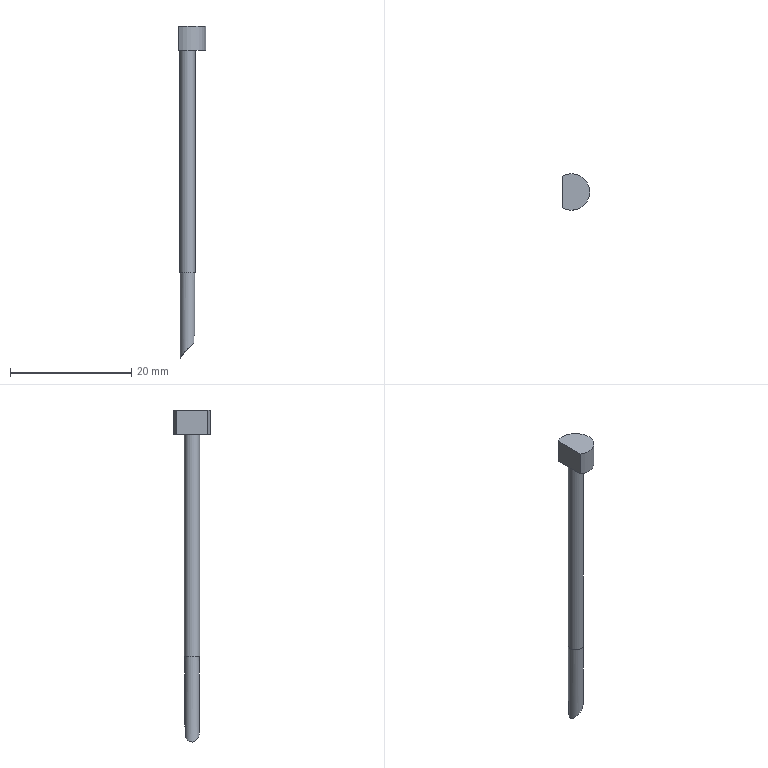Part | NX | features solid 2 | 1 solid | 10 faces | box 4.5 x 6 x 54.716 mm | volume 326.28 mm3 | cylinder 6 | plane 4 | commonest cylinder face diameters 24.622 x2 2.412 x1 2.5 x1 6 x1 26.633 x1
STEP:
#1=CARTESIAN_POINT('',(-10.383,6.106,66.5));
#2=VERTEX_POINT('',#1);
#3=CARTESIAN_POINT('',(-10.383,6.106,70.5));
#4=VERTEX_POINT('',#3);
#5=CARTESIAN_POINT('',(-10.383,6.106,66.5));
#6=DIRECTION('',(0.,0.,1.));
#7=VECTOR('',#6,1000.);
#8=LINE('',#5,#7);
#9=EDGE_CURVE('',#2,#4,#8,.T.);
#10=ORIENTED_EDGE('',*,*,#9,.F.);
#11=CARTESIAN_POINT('',(-10.383,11.303,66.5));
#12=VERTEX_POINT('',#11);
#13=CARTESIAN_POINT('',(-8.883,8.704,66.5));
#14=DIRECTION('',(0.,0.,-1.));
#15=DIRECTION('',(-1.,0.,0.));
#16=AXIS2_PLACEMENT_3D('',#13,#14,#15);
#17=CIRCLE('',#16,3.);
#18=EDGE_CURVE('',#12,#2,#17,.T.);
#19=ORIENTED_EDGE('',*,*,#18,.F.);
#20=CARTESIAN_POINT('',(-10.383,11.303,70.5));
#21=VERTEX_POINT('',#20);
#22=CARTESIAN_POINT('',(-10.383,11.303,66.5));
#23=DIRECTION('',(0.,0.,1.));
#24=VECTOR('',#23,1000.);
#25=LINE('',#22,#24);
#26=EDGE_CURVE('',#21,#12,#25,.F.);
#27=ORIENTED_EDGE('',*,*,#26,.F.);
#28=CARTESIAN_POINT('',(-8.883,8.704,70.5));
#29=DIRECTION('',(0.,0.,-1.));
#30=DIRECTION('',(-1.,0.,0.));
#31=AXIS2_PLACEMENT_3D('',#28,#29,#30);
#32=CIRCLE('',#31,3.);
#33=EDGE_CURVE('',#21,#4,#32,.T.);
#34=ORIENTED_EDGE('',*,*,#33,.T.);
#35=EDGE_LOOP('',(#10,#19,#27,#34));
#36=FACE_BOUND('',#35,.T.);
#37=CARTESIAN_POINT('',(-8.883,8.704,66.5));
#38=DIRECTION('',(0.,0.,1.));
#39=DIRECTION('',(1.,0.,0.));
#40=AXIS2_PLACEMENT_3D('',#37,#38,#39);
#41=CYLINDRICAL_SURFACE('',#40,3.);
#42=ADVANCED_FACE('',(#36),#41,.T.);
#43=CARTESIAN_POINT('',(-10.133,8.704,66.5));
#44=VERTEX_POINT('',#43);
#45=CARTESIAN_POINT('',(-8.883,8.704,66.5));
#46=DIRECTION('',(0.,0.,-1.));
#47=DIRECTION('',(-1.,0.,0.));
#48=AXIS2_PLACEMENT_3D('',#45,#46,#47);
#49=CIRCLE('',#48,1.25);
#50=EDGE_CURVE('',#44,#44,#49,.F.);
#51=ORIENTED_EDGE('',*,*,#50,.T.);
#52=EDGE_LOOP('',(#51));
#53=FACE_BOUND('',#52,.T.);
#54=ORIENTED_EDGE('',*,*,#18,.T.);
#55=CARTESIAN_POINT('',(-10.383,8.704,66.5));
#56=DIRECTION('',(0.,1.,0.));
#57=VECTOR('',#56,1000.);
#58=LINE('',#55,#57);
#59=EDGE_CURVE('',#2,#12,#58,.T.);
#60=ORIENTED_EDGE('',*,*,#59,.T.);
#61=EDGE_LOOP('',(#54,#60));
#62=FACE_BOUND('',#61,.T.);
#63=CARTESIAN_POINT('',(-8.883,8.704,66.5));
#64=DIRECTION('',(0.,0.,-1.));
#65=DIRECTION('',(-1.,0.,0.));
#66=AXIS2_PLACEMENT_3D('',#63,#64,#65);
#67=PLANE('',#66);
#68=ADVANCED_FACE('',(#53,#62),#67,.T.);
#69=ORIENTED_EDGE('',*,*,#33,.F.);
#70=CARTESIAN_POINT('',(-10.383,0.,70.5));
#71=DIRECTION('',(0.,-1.,0.));
#72=VECTOR('',#71,1000.);
#73=LINE('',#70,#72);
#74=EDGE_CURVE('',#4,#21,#73,.F.);
#75=ORIENTED_EDGE('',*,*,#74,.F.);
#76=EDGE_LOOP('',(#69,#75));
#77=FACE_BOUND('',#76,.T.);
#78=CARTESIAN_POINT('',(0.,0.,70.5));
#79=DIRECTION('',(0.,0.,1.));
#80=DIRECTION('',(1.,0.,0.));
#81=AXIS2_PLACEMENT_3D('',#78,#79,#80);
#82=PLANE('',#81);
#83=ADVANCED_FACE('',(#77),#82,.T.);
#84=CARTESIAN_POINT('',(-7.841,8.097,18.216));
#85=VERTEX_POINT('',#84);
#86=CARTESIAN_POINT('',(-9.491,9.746,16.567));
#87=VERTEX_POINT('',#86);
#88=CARTESIAN_POINT('',(-9.491,9.746,16.567));
#89=CARTESIAN_POINT('',(-9.233,9.434,16.878));
#90=CARTESIAN_POINT('',(-8.697,8.848,17.465));
#91=CARTESIAN_POINT('',(-8.13,8.335,17.978));
#92=CARTESIAN_POINT('',(-7.841,8.097,18.216));
#93=B_SPLINE_CURVE_WITH_KNOTS('',3,(#88,#89,#90,#91,#92),.UNSPECIFIED.,.F.,.F.,(4,1,4),(0.,0.5,1.),.QUASI_UNIFORM_KNOTS.);
#94=EDGE_CURVE('',#85,#87,#93,.F.);
#95=ORIENTED_EDGE('',*,*,#94,.F.);
#96=CARTESIAN_POINT('',(-9.491,9.746,16.567));
#97=CARTESIAN_POINT('',(-9.63,9.665,16.398));
#98=CARTESIAN_POINT('',(-9.883,9.453,16.074));
#99=CARTESIAN_POINT('',(-10.152,8.849,15.69));
#100=CARTESIAN_POINT('',(-10.004,8.124,15.905));
#101=CARTESIAN_POINT('',(-9.529,7.605,16.541));
#102=CARTESIAN_POINT('',(-8.763,7.374,17.415));
#103=CARTESIAN_POINT('',(-8.06,7.722,18.036));
#104=CARTESIAN_POINT('',(-7.841,8.097,18.216));
#105=B_SPLINE_CURVE_WITH_KNOTS('',3,(#96,#97,#98,#99,#100,#101,#102,#103,#104),.UNSPECIFIED.,.F.,.F.,(4,1,1,1,1,1,4),(0.,0.0006946,0.001389,0.002084,0.002778,0.004167,0.005557),.UNSPECIFIED.);
#106=EDGE_CURVE('',#85,#87,#105,.F.);
#107=ORIENTED_EDGE('',*,*,#106,.T.);
#108=EDGE_LOOP('',(#95,#107));
#109=FACE_BOUND('',#108,.T.);
#110=CARTESIAN_POINT('',(0.,-2.743,8.725));
#111=DIRECTION('',(0.,1.,0.));
#112=DIRECTION('',(-1.,0.,0.));
#113=AXIS2_PLACEMENT_3D('',#110,#111,#112);
#114=CYLINDRICAL_SURFACE('',#113,12.311);
#115=ADVANCED_FACE('',(#109),#114,.F.);
#116=CARTESIAN_POINT('',(-9.491,9.746,18.066));
#117=VERTEX_POINT('',#116);
#118=CARTESIAN_POINT('',(-7.841,8.097,19.488));
#119=VERTEX_POINT('',#118);
#120=CARTESIAN_POINT('',(-7.841,8.097,19.488));
#121=CARTESIAN_POINT('',(-8.131,8.336,19.277));
#122=CARTESIAN_POINT('',(-8.699,8.85,18.827));
#123=CARTESIAN_POINT('',(-9.234,9.435,18.327));
#124=CARTESIAN_POINT('',(-9.491,9.746,18.066));
#125=B_SPLINE_CURVE_WITH_KNOTS('',3,(#120,#121,#122,#123,#124),.UNSPECIFIED.,.F.,.F.,(4,1,4),(0.,0.5,1.),.QUASI_UNIFORM_KNOTS.);
#126=EDGE_CURVE('',#117,#119,#125,.F.);
#127=ORIENTED_EDGE('',*,*,#126,.F.);
#128=CARTESIAN_POINT('',(-8.883,9.91,18.646));
#129=VERTEX_POINT('',#128);
#130=CARTESIAN_POINT('',(-8.883,9.91,18.646));
#131=CARTESIAN_POINT('',(-8.926,9.91,18.607));
#132=CARTESIAN_POINT('',(-9.011,9.906,18.53));
#133=CARTESIAN_POINT('',(-9.136,9.886,18.413));
#134=CARTESIAN_POINT('',(-9.259,9.853,18.296));
#135=CARTESIAN_POINT('',(-9.377,9.807,18.18));
#136=CARTESIAN_POINT('',(-9.454,9.768,18.104));
#137=CARTESIAN_POINT('',(-9.491,9.746,18.066));
#138=B_SPLINE_CURVE_WITH_KNOTS('',3,(#130,#131,#132,#133,#134,#135,#136,#137),.UNSPECIFIED.,.F.,.F.,(4,1,1,1,1,4),(0.,0.2,0.4,0.6,0.8,1.),.QUASI_UNIFORM_KNOTS.);
#139=EDGE_CURVE('',#117,#129,#138,.F.);
#140=ORIENTED_EDGE('',*,*,#139,.T.);
#141=CARTESIAN_POINT('',(-7.841,8.097,19.488));
#142=CARTESIAN_POINT('',(-7.617,8.482,19.652));
#143=CARTESIAN_POINT('',(-7.721,9.603,19.587));
#144=CARTESIAN_POINT('',(-8.531,9.91,18.961));
#145=CARTESIAN_POINT('',(-8.883,9.91,18.646));
#146=B_SPLINE_CURVE_WITH_KNOTS('',3,(#141,#142,#143,#144,#145),.UNSPECIFIED.,.F.,.F.,(4,1,4),(0.,0.001408,0.002815),.UNSPECIFIED.);
#147=EDGE_CURVE('',#129,#119,#146,.F.);
#148=ORIENTED_EDGE('',*,*,#147,.T.);
#149=EDGE_LOOP('',(#127,#140,#148));
#150=FACE_BOUND('',#149,.T.);
#151=CARTESIAN_POINT('',(0.,0.,8.725));
#152=DIRECTION('',(0.,-1.,0.));
#153=DIRECTION('',(1.,0.,0.));
#154=AXIS2_PLACEMENT_3D('',#151,#152,#153);
#155=CYLINDRICAL_SURFACE('',#154,13.316);
#156=ADVANCED_FACE('',(#150),#155,.F.);
#157=CARTESIAN_POINT('',(-9.491,9.746,16.567));
#158=DIRECTION('',(0.,0.,1.));
#159=VECTOR('',#158,1000.);
#160=LINE('',#157,#159);
#161=EDGE_CURVE('',#87,#117,#160,.T.);
#162=ORIENTED_EDGE('',*,*,#161,.T.);
#163=ORIENTED_EDGE('',*,*,#126,.T.);
#164=CARTESIAN_POINT('',(-7.841,8.097,18.216));
#165=DIRECTION('',(0.,0.,1.));
#166=VECTOR('',#165,1000.);
#167=LINE('',#164,#166);
#168=EDGE_CURVE('',#119,#85,#167,.F.);
#169=ORIENTED_EDGE('',*,*,#168,.T.);
#170=ORIENTED_EDGE('',*,*,#94,.T.);
#171=EDGE_LOOP('',(#162,#163,#169,#170));
#172=FACE_BOUND('',#171,.T.);
#173=CARTESIAN_POINT('',(0.,17.587,31.84));
#174=DIRECTION('',(0.,0.,1.));
#175=DIRECTION('',(0.,-1.,0.));
#176=AXIS2_PLACEMENT_3D('',#173,#174,#175);
#177=CYLINDRICAL_SURFACE('',#176,12.311);
#178=ADVANCED_FACE('',(#172),#177,.F.);
#179=ORIENTED_EDGE('',*,*,#168,.F.);
#180=ORIENTED_EDGE('',*,*,#147,.F.);
#181=ORIENTED_EDGE('',*,*,#139,.F.);
#182=ORIENTED_EDGE('',*,*,#161,.F.);
#183=ORIENTED_EDGE('',*,*,#106,.F.);
#184=EDGE_LOOP('',(#179,#180,#181,#182,#183));
#185=FACE_BOUND('',#184,.T.);
#186=CARTESIAN_POINT('',(-8.883,9.91,29.83));
#187=VERTEX_POINT('',#186);
#188=CARTESIAN_POINT('',(-8.883,8.704,29.83));
#189=DIRECTION('',(0.,0.,1.));
#190=DIRECTION('',(0.,1.,0.));
#191=AXIS2_PLACEMENT_3D('',#188,#189,#190);
#192=CIRCLE('',#191,1.206);
#193=EDGE_CURVE('',#187,#187,#192,.F.);
#194=ORIENTED_EDGE('',*,*,#193,.T.);
#195=EDGE_LOOP('',(#194));
#196=FACE_BOUND('',#195,.T.);
#197=CARTESIAN_POINT('',(-8.883,8.704,31.84));
#198=DIRECTION('',(0.,0.,1.));
#199=DIRECTION('',(0.,-1.,0.));
#200=AXIS2_PLACEMENT_3D('',#197,#198,#199);
#201=CYLINDRICAL_SURFACE('',#200,1.206);
#202=ADVANCED_FACE('',(#185,#196),#201,.T.);
#203=CARTESIAN_POINT('',(-7.633,8.704,29.83));
#204=VERTEX_POINT('',#203);
#205=CARTESIAN_POINT('',(-8.883,8.704,29.83));
#206=DIRECTION('',(0.,0.,1.));
#207=DIRECTION('',(1.,0.,0.));
#208=AXIS2_PLACEMENT_3D('',#205,#206,#207);
#209=CIRCLE('',#208,1.25);
#210=EDGE_CURVE('',#204,#204,#209,.F.);
#211=ORIENTED_EDGE('',*,*,#210,.T.);
#212=EDGE_LOOP('',(#211));
#213=FACE_BOUND('',#212,.T.);
#214=ORIENTED_EDGE('',*,*,#193,.F.);
#215=EDGE_LOOP('',(#214));
#216=FACE_BOUND('',#215,.T.);
#217=CARTESIAN_POINT('',(0.,0.,29.83));
#218=DIRECTION('',(0.,0.,1.));
#219=DIRECTION('',(0.,-1.,0.));
#220=AXIS2_PLACEMENT_3D('',#217,#218,#219);
#221=PLANE('',#220);
#222=ADVANCED_FACE('',(#213,#216),#221,.F.);
#223=ORIENTED_EDGE('',*,*,#50,.F.);
#224=EDGE_LOOP('',(#223));
#225=FACE_BOUND('',#224,.T.);
#226=ORIENTED_EDGE('',*,*,#210,.F.);
#227=EDGE_LOOP('',(#226));
#228=FACE_BOUND('',#227,.T.);
#229=CARTESIAN_POINT('',(-8.883,8.704,108.83));
#230=DIRECTION('',(0.,0.,-1.));
#231=DIRECTION('',(-1.,0.,0.));
#232=AXIS2_PLACEMENT_3D('',#229,#230,#231);
#233=CYLINDRICAL_SURFACE('',#232,1.25);
#234=ADVANCED_FACE('',(#225,#228),#233,.T.);
#235=ORIENTED_EDGE('',*,*,#59,.F.);
#236=ORIENTED_EDGE('',*,*,#9,.T.);
#237=ORIENTED_EDGE('',*,*,#74,.T.);
#238=ORIENTED_EDGE('',*,*,#26,.T.);
#239=EDGE_LOOP('',(#235,#236,#237,#238));
#240=FACE_BOUND('',#239,.T.);
#241=CARTESIAN_POINT('',(-10.383,17.587,43.14));
#242=DIRECTION('',(-1.,0.,0.));
#243=DIRECTION('',(0.,0.,1.));
#244=AXIS2_PLACEMENT_3D('',#241,#242,#243);
#245=PLANE('',#244);
#246=ADVANCED_FACE('',(#240),#245,.T.);
#247=CLOSED_SHELL('',(#42,#68,#83,#115,#156,#178,#202,#222,#234,#246));
#248=MANIFOLD_SOLID_BREP('',#247);
#249=(LENGTH_UNIT()NAMED_UNIT(*)SI_UNIT(.MILLI.,.METRE.));
#250=UNCERTAINTY_MEASURE_WITH_UNIT(LENGTH_MEASURE(0.0508),#249,'','');
#251=(NAMED_UNIT(*)PLANE_ANGLE_UNIT()SI_UNIT($,.RADIAN.));
#252=(NAMED_UNIT(*)SI_UNIT($,.STERADIAN.)SOLID_ANGLE_UNIT());
#253=(GEOMETRIC_REPRESENTATION_CONTEXT(3)GLOBAL_UNCERTAINTY_ASSIGNED_CONTEXT((#250))GLOBAL_UNIT_ASSIGNED_CONTEXT((#249,#251,#252))REPRESENTATION_CONTEXT('',''));
#254=ADVANCED_BREP_SHAPE_REPRESENTATION('',(#248),#253);